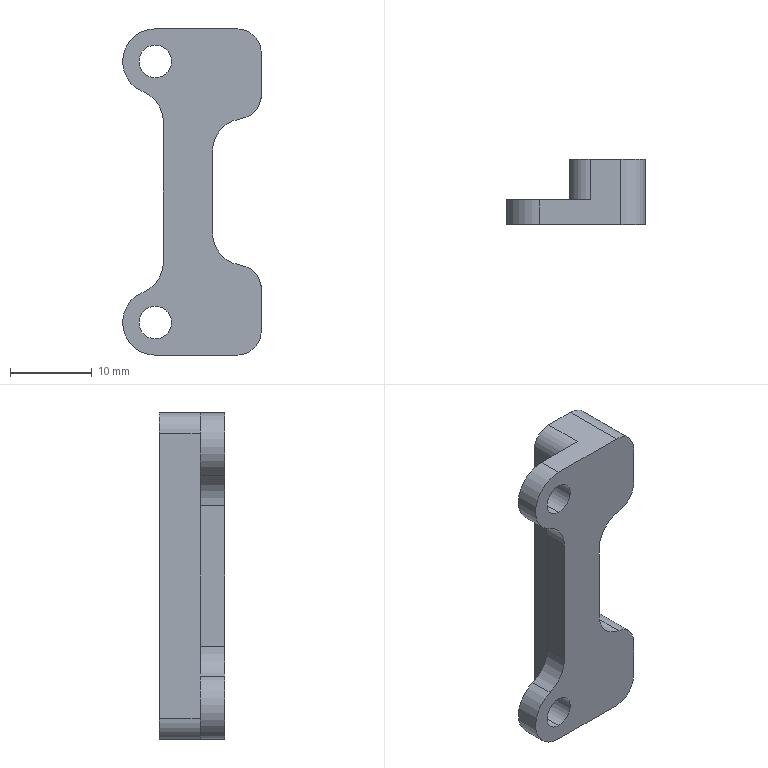NC program | Mastercam | posted with a generic post | part box 17 x 8 x 40 mm
Lines 25 to 1287 of 8055:
(8 FEM |TOOL - 8|DIA. OFF. - 8|LEN. - 8|TOOL DIA. - 8.)
N134 T8 M6
N136 G0 G54 G90 X-27.234 Y-18.253 C0. B0. S7000 M3
N138 G43 H8 Z50.
N140 Z3.
N142 G1 Z-8.25 F600.
N144 X-27.475 Y-17.573 Z-8.368 F3000.
N146 G3 X-27.899 Y-16.899 Z-8.5 I-1.697 J-.599
N148 G1 X-28.108 Y-16.578
N150 X-28.311 Y-16.174
N152 X-28.477 Y-15.79
N154 X-28.607 Y-15.435
N156 X-28.705 Y-15.109
N158 X-28.778 Y-14.809
N160 X-28.832 Y-14.534
N162 X-28.872 Y-14.281
N164 X-28.925 Y-13.837
N166 X-28.957 Y-13.437
N168 X-28.976 Y-13.068
N170 X-28.987 Y-12.722
N172 X-28.993 Y-12.392
N174 X-28.997 Y-12.073
N176 X-28.998 Y-11.761
N178 Y-11.455
N180 X-28.997 Y-11.151
N182 X-28.996 Y-10.85
N184 X-28.995 Y-10.55
N186 X-28.993 Y-10.251
N188 X-28.991 Y-9.952
N190 X-28.989 Y-9.653
N192 X-28.987 Y-9.355
N194 X-28.985 Y-9.056
N196 X-28.983 Y-8.757
N198 X-28.981 Y-8.459
N200 X-28.979 Y-8.16
N202 X-28.977 Y-7.862
N204 X-28.975 Y-7.563
N206 X-28.973 Y-7.264
N208 X-28.971 Y-6.965
N210 X-28.969 Y-6.666
N212 X-28.967 Y-6.367
N214 X-28.965 Y-6.068
N216 X-28.963 Y-5.769
N218 X-28.961 Y-5.47
N220 X-28.958 Y-5.171
N222 X-28.956 Y-4.872
N224 X-28.954 Y-4.573
N226 X-28.952 Y-4.273
N228 X-28.95 Y-3.974
N230 X-28.948 Y-3.674
N232 X-28.946 Y-3.375
N234 X-28.944 Y-3.075
N236 X-28.942 Y-2.776
N238 X-28.94 Y-2.476
N240 X-28.938 Y-2.176
N242 X-28.936 Y-1.877
N244 X-28.934 Y-1.577
N246 X-28.932 Y-1.277
N248 X-28.93 Y-.977
N250 X-28.928 Y-.677
N252 X-28.926 Y-.377
N254 X-28.924 Y-.077
N256 X-28.921 Y.223
N258 X-28.919 Y.523
N260 X-28.917 Y.823
N262 X-28.915 Y1.123
N264 X-28.913 Y1.423
N266 X-28.911 Y1.724
N268 X-28.909 Y2.024
N270 X-28.907 Y2.324
N272 X-28.905 Y2.625
N274 X-28.903 Y2.925
N276 X-28.901 Y3.225
N278 X-28.899 Y3.526
N280 X-28.897 Y3.826
N282 X-28.895 Y4.127
N284 X-28.893 Y4.428
N286 X-28.891 Y4.728
N288 X-28.888 Y5.029
N290 X-28.886 Y5.329
N292 X-28.884 Y5.63
N294 X-28.882 Y5.931
N296 X-28.88 Y6.232
N298 X-28.878 Y6.532
N300 X-28.876 Y6.833
N302 X-28.874 Y7.134
N304 X-28.872 Y7.435
N306 X-28.87 Y7.736
N308 X-28.868 Y8.037
N310 X-28.866 Y8.338
N312 X-28.864 Y8.639
N314 X-28.862 Y8.94
N316 X-28.86 Y9.241
N318 X-28.858 Y9.542
N320 X-28.855 Y9.843
N322 X-28.853 Y10.144
N324 X-28.851 Y10.445
N326 X-28.849 Y10.746
N328 X-28.847 Y11.047
N330 X-28.845 Y11.348
N332 X-28.843 Y11.65
N334 X-28.841 Y11.951
N336 X-28.839 Y12.252
N338 X-28.837 Y12.554
N340 X-28.829 Y12.843
N342 X-28.792 Y13.204
N344 X-28.72 Y13.565
N346 X-28.614 Y13.921
N348 X-28.475 Y14.267
N350 X-28.308 Y14.598
N352 X-28.116 Y14.911
N354 X-27.903 Y15.204
N356 X-27.674 Y15.473
N358 X-27.432 Y15.72
N360 X-27.181 Y15.944
N362 X-26.925 Y16.145
N364 X-26.666 Y16.326
N366 X-26.408 Y16.487
N368 X-26.15 Y16.629
N370 X-25.896 Y16.756
N372 X-25.646 Y16.867
N374 X-25.401 Y16.966
N376 X-25.161 Y17.052
N378 X-24.926 Y17.128
N380 X-24.697 Y17.195
N382 X-24.263 Y17.305
N384 X-23.847 Y17.392
N386 X-23.447 Y17.46
N388 X-23.062 Y17.514
N390 X-22.69 Y17.556
N392 X-22.329 Y17.59
N394 X-21.978 Y17.617
N396 X-21.635 Y17.638
N398 X-21.299 Y17.654
N400 X-20.968 Y17.667
N402 X-20.643 Y17.678
N404 X-20.322 Y17.685
N406 X-20.004 Y17.691
N408 X-19.689 Y17.696
N410 X-19.377 Y17.699
N412 X-19.066 Y17.701
N414 X-18.757 Y17.702
N416 X-18.449
N418 X-18.143
N420 X-17.837
N422 X-17.533 Y17.701
N424 X-17.228 Y17.7
N426 X-16.924 Y17.698
N428 X-16.621 Y17.697
N430 X-16.317 Y17.695
N432 X-16.014 Y17.693
N434 X-15.711 Y17.692
N436 X-15.408 Y17.69
N438 X-15.105 Y17.688
N440 X-14.803 Y17.686
N442 X-14.5 Y17.684
N444 X-14.197 Y17.682
N446 X-13.895 Y17.68
N448 X-13.592 Y17.678
N450 X-13.289 Y17.676
N452 X-12.987 Y17.674
N454 X-12.684 Y17.672
N456 X-12.381 Y17.67
N458 X-12.079 Y17.668
N460 X-11.776 Y17.665
N462 X-11.473 Y17.663
N464 X-11.171 Y17.661
N466 X-10.868 Y17.659
N468 X-10.565 Y17.657
N470 X-10.263 Y17.655
N472 X-9.96 Y17.653
N474 X-9.657 Y17.651
N476 X-9.354 Y17.649
N478 X-9.052 Y17.647
N480 X-8.749 Y17.645
N482 X-8.446 Y17.643
N484 X-8.143 Y17.641
N486 X-7.841 Y17.638
N488 X-7.538 Y17.636
N490 X-7.235 Y17.634
N492 X-6.932 Y17.632
N494 X-6.629 Y17.63
N496 X-6.327 Y17.628
N498 X-6.024 Y17.626
N500 X-5.721 Y17.624
N502 X-5.418 Y17.622
N504 X-5.115 Y17.62
N506 X-4.812 Y17.618
N508 X-4.509 Y17.616
N510 X-4.206 Y17.614
N512 X-3.903 Y17.612
N514 X-3.599 Y17.61
N516 X-3.295 Y17.608
N518 X-2.99 Y17.607
N520 X-2.685 Y17.606
N522 X-2.38 Y17.605
N524 X-2.075 Y17.604
N526 X-1.769
N528 X-1.463 Y17.603
N530 X-1.157
N532 X-.851 Y17.602
N534 X-.545
N536 X-.239
N538 X.067 Y17.601
N540 X.374
N542 X.68
N544 X.986
N546 X1.293
N548 X1.6
N550 X1.906
N552 X2.213 Y17.6
N554 X2.519
N556 X2.826
N558 X3.133
N560 X3.439
N562 X3.746
N564 X4.053
N566 X4.359
N568 X4.666
N570 X4.973
N572 X5.279
N574 X5.586
N576 X5.893
N578 X6.199
N580 X6.506
N582 X6.813
N584 X7.12
N586 X7.426
N588 X7.733
N590 X8.04
N592 X8.346
N594 X8.653
N596 X8.96
N598 X9.267
N600 X9.573
N602 X9.88
N604 X10.187
N606 X10.493
N608 X10.8
N610 X11.107
N612 X11.414
N614 X11.72
N616 X12.027
N618 X12.334
N620 X12.641
N622 X12.947
N624 X13.254
N626 X13.561
N628 X13.867
N630 X14.174
N632 X14.481
N634 X14.788
N636 X15.094
N638 X15.401
N640 X15.708
N642 X16.015
N644 X16.321
N646 X16.628
N648 X16.935
N650 X17.241
N652 X17.548
N654 X17.855
N656 X18.162
N658 X18.468
N660 X18.775
N662 X19.082
N664 X19.389
N666 X19.695
N668 X20.002
N670 X20.309
N672 X20.616
N674 X20.922
N676 X21.229
N678 X21.536
N680 X21.842
N682 X22.149
N684 X22.456
N686 X22.763
N688 X23.07
N690 X23.335 Y17.595
N692 X23.605 Y17.572
N694 X23.881 Y17.527
N696 X24.16 Y17.461
N698 X24.439 Y17.374
N700 X24.714 Y17.266
N702 X24.984 Y17.138
N704 X25.246 Y16.992
N706 X25.497 Y16.83
N708 X25.737 Y16.653
N710 X25.965 Y16.463
N712 X26.179 Y16.263
N714 X26.38 Y16.054
N716 X26.567 Y15.839
N718 X26.74 Y15.619
N720 X26.901 Y15.395
N722 X27.048 Y15.168
N724 X27.183 Y14.941
N726 X27.308 Y14.713
N728 X27.421 Y14.487
N730 X27.525 Y14.261
N732 X27.619 Y14.037
N734 X27.705 Y13.816
N736 X27.852 Y13.388
N738 X27.975 Y12.971
N740 X28.076 Y12.564
N742 X28.161 Y12.168
N744 X28.231 Y11.782
N746 X28.29 Y11.405
N748 X28.339 Y11.037
N750 X28.38 Y10.677
N752 X28.414 Y10.324
N754 X28.443 Y9.978
N756 X28.467 Y9.637
N758 X28.487 Y9.3
N760 X28.504 Y8.968
N762 X28.519 Y8.639
N764 X28.531 Y8.314
N766 X28.541 Y7.991
N768 X28.55 Y7.67
N770 X28.557 Y7.351
N772 X28.564 Y7.035
N774 X28.569 Y6.719
N776 X28.574 Y6.405
N778 X28.578 Y6.092
N780 X28.581 Y5.78
N782 X28.584 Y5.468
N784 X28.586 Y5.158
N786 X28.588 Y4.848
N788 X28.59 Y4.538
N790 X28.591 Y4.229
N792 X28.593 Y3.92
N794 X28.594 Y3.611
N796 X28.595 Y3.303
N798 Y2.995
N800 X28.596 Y2.687
N802 X28.597 Y2.38
N804 Y2.072
N806 X28.598 Y1.765
N808 Y1.457
N810 Y1.15
N812 X28.599 Y.843
N814 Y.536
N816 Y.229
N818 Y-.078
N820 Y-.385
N822 Y-.692
N824 Y-.999
N826 X28.6 Y-1.306
N828 Y-1.613
N830 Y-1.92
N832 Y-2.226
N834 Y-2.533
N836 Y-2.84
N838 Y-3.147
N840 Y-3.454
N842 Y-3.76
N844 Y-4.067
N846 Y-4.374
N848 Y-4.681
N850 Y-4.987
N852 Y-5.294
N854 Y-5.601
N856 Y-5.908
N858 Y-6.214
N860 Y-6.521
N862 Y-6.828
N864 Y-7.135
N866 Y-7.441
N868 Y-7.748
N870 Y-8.055
N872 Y-8.361
N874 Y-8.668
N876 Y-8.975
N878 Y-9.282
N880 Y-9.588
N882 Y-9.895
N884 Y-10.202
N886 Y-10.509
N888 Y-10.815
N890 Y-11.122
N892 Y-11.429
N894 Y-11.736
N896 Y-12.042
N898 X28.597 Y-12.286
N900 X28.577 Y-12.558
N902 X28.536 Y-12.834
N904 X28.474 Y-13.112
N906 X28.391 Y-13.391
N908 X28.286 Y-13.667
N910 X28.161 Y-13.938
N912 X28.018 Y-14.201
N914 X27.859 Y-14.455
N916 X27.684 Y-14.697
N918 X27.497 Y-14.927
N920 X27.298 Y-15.143
N922 X27.091 Y-15.346
N924 X26.877 Y-15.536
N926 X26.657 Y-15.711
N928 X26.433 Y-15.874
N930 X26.207 Y-16.024
N932 X25.98 Y-16.161
N934 X25.753 Y-16.287
N936 X25.526 Y-16.402
N938 X25.3 Y-16.507
N940 X25.076 Y-16.603
N942 X24.854 Y-16.691
N944 X24.425 Y-16.84
N946 X24.007 Y-16.965
N948 X23.599 Y-17.068
N950 X23.202 Y-17.154
N952 X22.815 Y-17.226
N954 X22.438 Y-17.285
N956 X22.069 Y-17.335
N958 X21.709 Y-17.376
N960 X21.355 Y-17.411
N962 X21.008 Y-17.44
N964 X20.666 Y-17.465
N966 X20.329 Y-17.485
N968 X19.997 Y-17.503
N970 X19.668 Y-17.517
N972 X19.342 Y-17.53
N974 X19.019 Y-17.54
N976 X18.698 Y-17.549
N978 X18.379 Y-17.557
N980 X18.062 Y-17.563
N982 X17.747 Y-17.569
N984 X17.433 Y-17.573
N986 X17.119 Y-17.577
N988 X16.807 Y-17.581
N990 X16.496 Y-17.584
N992 X16.185 Y-17.586
N994 X15.875 Y-17.588
N996 X15.565 Y-17.59
N998 X15.256 Y-17.591
N1000 X14.947 Y-17.593
N1002 X14.638 Y-17.594
N1004 X14.33 Y-17.595
N1006 X14.022
N1008 X13.714 Y-17.596
N1010 X13.407 Y-17.597
N1012 X13.099
N1014 X12.792 Y-17.598
N1016 X12.484
N1018 X12.177
N1020 X11.87
N1022 X11.563 Y-17.599
N1024 X11.256
N1026 X10.949
N1028 X10.642
N1030 X10.335
N1032 X10.028
N1034 X9.721 Y-17.6
N1036 X9.414
N1038 X9.107
N1040 X8.801
N1042 X8.494
N1044 X8.187
N1046 X7.88
N1048 X7.573
N1050 X7.267
N1052 X6.96
N1054 X6.653
N1056 X6.346
N1058 X6.04
N1060 X5.733
N1062 X5.426
N1064 X5.119
N1066 X4.813
N1068 X4.506
N1070 X4.199
N1072 X3.892
N1074 X3.586
N1076 X3.279
N1078 X2.972
N1080 X2.665
N1082 X2.359
N1084 X2.052
N1086 X1.745
N1088 X1.439
N1090 X1.132
N1092 X.825
N1094 X.518
N1096 X.212
N1098 X-.095
N1100 X-.402
N1102 X-.709
N1104 X-1.015
N1106 X-1.322
N1108 X-1.629
N1110 X-1.936
N1112 X-2.242
N1114 X-2.549
N1116 X-2.856
N1118 X-3.162
N1120 X-3.469
N1122 X-3.776
N1124 X-4.083
N1126 X-4.389
N1128 X-4.696
N1130 X-5.003
N1132 X-5.31
N1134 X-5.616
N1136 X-5.923
N1138 X-6.23
N1140 X-6.536
N1142 X-6.843
N1144 X-7.15
N1146 X-7.457
N1148 X-7.763
N1150 X-8.07
N1152 X-8.377
N1154 X-8.684
N1156 X-8.99
N1158 X-9.297
N1160 X-9.604
N1162 X-9.91
N1164 X-10.217
N1166 X-10.524
N1168 X-10.831
N1170 X-11.137
N1172 X-11.444
N1174 X-11.751
N1176 X-12.058
N1178 X-12.364
N1180 X-12.671
N1182 X-12.978
N1184 X-13.284
N1186 X-13.591
N1188 X-13.898
N1190 X-14.205
N1192 X-14.511
N1194 X-14.818
N1196 X-15.125
N1198 X-15.432
N1200 X-15.738
N1202 X-16.045
N1204 X-16.352
N1206 X-16.658
N1208 X-16.965
N1210 X-17.272
N1212 X-17.579
N1214 X-17.885
N1216 X-18.192
N1218 X-18.499
N1220 X-18.806
N1222 X-19.112
N1224 X-19.419
N1226 X-19.726
N1228 X-20.033
N1230 X-20.339
N1232 X-20.646
N1234 X-20.953
N1236 X-21.259
N1238 X-21.566
N1240 X-21.873
N1242 X-22.18
N1244 X-22.486
N1246 X-22.793
N1248 X-22.993 Y-17.599
N1250 X-23.283 Y-17.582
N1252 X-23.573 Y-17.543
N1254 X-23.86 Y-17.485
N1256 X-24.146 Y-17.405
N1258 X-24.427 Y-17.306
N1260 X-24.702 Y-17.187
N1262 X-24.969 Y-17.051
N1264 X-25.226 Y-16.898
N1266 X-25.473 Y-16.73
N1268 X-25.708 Y-16.549
N1270 X-25.93 Y-16.357
N1272 X-26.139 Y-16.154
N1274 X-26.335 Y-15.944
N1276 X-26.517 Y-15.728
N1278 X-26.686 Y-15.507
N1280 X-26.842 Y-15.282
N1282 X-26.986 Y-15.055
N1284 X-27.118 Y-14.828
N1286 X-27.24 Y-14.6
N1288 X-27.35 Y-14.373
N1290 X-27.451 Y-14.147
N1292 X-27.543 Y-13.924
N1294 X-27.627 Y-13.702
N1296 X-27.77 Y-13.274
N1298 X-27.889 Y-12.856
N1300 X-27.987 Y-12.449
N1302 X-28.069 Y-12.053
N1304 X-28.136 Y-11.667
N1306 X-28.192 Y-11.29
N1308 X-28.238 Y-10.922
N1310 X-28.276 Y-10.562
N1312 X-28.308 Y-10.21
N1314 X-28.334 Y-9.863
N1316 X-28.356 Y-9.522
N1318 X-28.374 Y-9.185
N1320 X-28.388 Y-8.853
N1322 X-28.4 Y-8.524
N1324 X-28.41 Y-8.198
N1326 X-28.419 Y-7.876
N1328 X-28.425 Y-7.555
N1330 X-28.43 Y-7.236
N1332 X-28.434 Y-6.919
N1334 X-28.438 Y-6.604
N1336 X-28.44 Y-6.29
N1338 X-28.442 Y-5.977
N1340 X-28.443 Y-5.665
N1342 X-28.444 Y-5.353
N1344 Y-5.043
N1346 Y-4.733
N1348 X-28.443 Y-4.423
N1350 Y-4.114
N1352 X-28.442 Y-3.805
N1354 X-28.441 Y-3.496
N1356 X-28.44 Y-3.188
N1358 X-28.438 Y-2.88
N1360 X-28.437 Y-2.572
N1362 X-28.435 Y-2.265
N1364 X-28.434 Y-1.957
N1366 X-28.432 Y-1.65
N1368 X-28.43 Y-1.342
N1370 X-28.428 Y-1.035
N1372 X-28.426 Y-.728
N1374 X-28.425 Y-.421
N1376 X-28.423 Y-.114
N1378 X-28.421 Y.193
N1380 X-28.419 Y.5
N1382 X-28.417 Y.807
N1384 X-28.415 Y1.114
N1386 X-28.413 Y1.421
N1388 X-28.411 Y1.728
N1390 X-28.409 Y2.034
N1392 X-28.407 Y2.341
N1394 X-28.405 Y2.648
N1396 X-28.402 Y2.955
N1398 X-28.4 Y3.262
N1400 X-28.398 Y3.568
N1402 X-28.396 Y3.875
N1404 X-28.394 Y4.182
N1406 X-28.392 Y4.489
N1408 X-28.39 Y4.795
N1410 X-28.388 Y5.102
N1412 X-28.386 Y5.409
N1414 X-28.384 Y5.716
N1416 X-28.382 Y6.022
N1418 X-28.379 Y6.329
N1420 X-28.377 Y6.636
N1422 X-28.375 Y6.943
N1424 X-28.373 Y7.249
N1426 X-28.371 Y7.556
N1428 X-28.369 Y7.863
N1430 X-28.367 Y8.169
N1432 X-28.365 Y8.476
N1434 X-28.363 Y8.783
N1436 X-28.361 Y9.09
N1438 X-28.358 Y9.396
N1440 X-28.356 Y9.703
N1442 X-28.354 Y10.01
N1444 X-28.352 Y10.317
N1446 X-28.35 Y10.625
N1448 X-28.347 Y10.838
N1450 X-28.333 Y11.114
N1452 X-28.305 Y11.399
N1454 X-28.262 Y11.687
N1456 X-28.203 Y11.974
N1458 X-28.127 Y12.258
N1460 X-28.036 Y12.537
N1462 X-27.93 Y12.81
N1464 X-27.809 Y13.077
N1466 X-27.674 Y13.335
N1468 X-27.526 Y13.585
N1470 X-27.368 Y13.824
N1472 X-27.198 Y14.054
N1474 X-27.019 Y14.273
N1476 X-26.831 Y14.481
N1478 X-26.637 Y14.678
N1480 X-26.436 Y14.864
N1482 X-26.231 Y15.039
N1484 X-26.021 Y15.203
N1486 X-25.809 Y15.356
N1488 X-25.594 Y15.5
N1490 X-25.377 Y15.633
N1492 X-25.16 Y15.757
N1494 X-24.942 Y15.872
N1496 X-24.725 Y15.978
N1498 X-24.509 Y16.077
N1500 X-24.087 Y16.249
N1502 X-23.67 Y16.396
N1504 X-23.261 Y16.521
N1506 X-22.859 Y16.628
N1508 X-22.465 Y16.717
N1510 X-22.08 Y16.793
N1512 X-21.702 Y16.857
N1514 X-21.331 Y16.911
N1516 X-20.968 Y16.957
N1518 X-20.611 Y16.995
N1520 X-20.26 Y17.027
N1522 X-19.915 Y17.054
N1524 X-19.574 Y17.077
N1526 X-19.238 Y17.096
N1528 X-18.905 Y17.111
N1530 X-18.576 Y17.124
N1532 X-18.25 Y17.135
N1534 X-17.926 Y17.144
N1536 X-17.605 Y17.151
N1538 X-17.286 Y17.157
N1540 X-16.969 Y17.161
N1542 X-16.653 Y17.165
N1544 X-16.338 Y17.168
N1546 X-16.024 Y17.17
N1548 X-15.712 Y17.171
N1550 X-15.4 Y17.172
N1552 X-15.089 Y17.173
N1554 X-14.779
N1556 X-14.469
N1558 X-14.159 Y17.172
N1560 X-13.85
N1562 X-13.542 Y17.171
N1564 X-13.233 Y17.17
N1566 X-12.925 Y17.168
N1568 X-12.617 Y17.167
N1570 X-12.309 Y17.165
N1572 X-12.002 Y17.164
N1574 X-11.694 Y17.162
N1576 X-11.387 Y17.161
N1578 X-11.08 Y17.159
N1580 X-10.772 Y17.157
N1582 X-10.465 Y17.155
N1584 X-10.158 Y17.153
N1586 X-9.851 Y17.151
N1588 X-9.544 Y17.149
N1590 X-9.237 Y17.147
N1592 X-8.93 Y17.145
N1594 X-8.623 Y17.143
N1596 X-8.317 Y17.141
N1598 X-8.01 Y17.139
N1600 X-7.703 Y17.137
N1602 X-7.396 Y17.135
N1604 X-7.089 Y17.133
N1606 X-6.782 Y17.131
N1608 X-6.476 Y17.129
N1610 X-6.169 Y17.127
N1612 X-5.862 Y17.125
N1614 X-5.556 Y17.123
N1616 X-5.25 Y17.121
N1618 X-4.945 Y17.119
N1620 X-4.639 Y17.117
N1622 X-4.334 Y17.115
N1624 X-4.028 Y17.114
N1626 X-3.723 Y17.112
N1628 X-3.417 Y17.111
N1630 X-3.112 Y17.11
N1632 X-2.806 Y17.109
N1634 X-2.5 Y17.108
N1636 X-2.195 Y17.107
N1638 X-1.889 Y17.106
N1640 X-1.583
N1642 X-1.277 Y17.105
N1644 X-.971 Y17.104
N1646 X-.665
N1648 X-.359 Y17.103
N1650 X-.052
N1652 X.254
N1654 X.56 Y17.102
N1656 X.866
N1658 X1.173
N1660 X1.479
N1662 X1.786 Y17.101
N1664 X2.092
N1666 X2.399
N1668 X2.705
N1670 X3.012
N1672 X3.318
N1674 X3.625
N1676 X3.932
N1678 X4.238 Y17.1
N1680 X4.545
N1682 X4.852
N1684 X5.158
N1686 X5.465
N1688 X5.772
N1690 X6.078
N1692 X6.385
N1694 X6.692
N1696 X6.998
N1698 X7.305
N1700 X7.612
N1702 X7.919
N1704 X8.225
N1706 X8.532
N1708 X8.839
N1710 X9.145
N1712 X9.452
N1714 X9.759
N1716 X10.066
N1718 X10.372
N1720 X10.679
N1722 X10.986
N1724 X11.292
N1726 X11.599
N1728 X11.906
N1730 X12.213
N1732 X12.519
N1734 X12.826
N1736 X13.133
N1738 X13.439
N1740 X13.746
N1742 X14.053
N1744 X14.36
N1746 X14.666
N1748 X14.973
N1750 X15.28
N1752 X15.587
N1754 X15.893
N1756 X16.2
N1758 X16.507
N1760 X16.813
N1762 X17.12
N1764 X17.427
N1766 X17.734
N1768 X18.04
N1770 X18.347
N1772 X18.654
N1774 X18.961
N1776 X19.267
N1778 X19.574
N1780 X19.881
N1782 X20.187
N1784 X20.494
N1786 X20.801
N1788 X21.108
N1790 X21.319 Y17.099
N1792 X21.591 Y17.088
N1794 X21.872 Y17.063
N1796 X22.155 Y17.025
N1798 X22.438 Y16.971
N1800 X22.72 Y16.903
N1802 X22.997 Y16.82
N1804 X23.269 Y16.723
N1806 X23.535 Y16.612
N1808 X23.794 Y16.489
N1810 X24.045 Y16.352
N1812 X24.287 Y16.205
N1814 X24.521 Y16.047
N1816 X24.744 Y15.881
N1818 X24.958 Y15.705
N1820 X25.161 Y15.523
N1822 X25.355 Y15.334
N1824 X25.538 Y15.139
N1826 X25.712 Y14.94
N1828 X25.875 Y14.737
N1830 X26.029 Y14.531
N1832 X26.174 Y14.323
N1834 X26.309 Y14.113
N1836 X26.436 Y13.902
N1838 X26.554 Y13.69
N1840 X26.665 Y13.478
N1842 X26.86 Y13.064
N1844 X27.03 Y12.652
N1846 X27.177 Y12.245
N1848 X27.305 Y11.844
N1850 X27.414 Y11.449
N1852 X27.509 Y11.061
N1854 X27.59 Y10.68
N1856 X27.66 Y10.306
N1858 X27.72 Y9.938
N1860 X27.772 Y9.576
N1862 X27.817 Y9.22
N1864 X27.855 Y8.869
N1866 X27.888 Y8.524
N1868 X27.917 Y8.182
N1870 X27.942 Y7.845
N1872 X27.963 Y7.511
N1874 X27.982 Y7.18
N1876 X27.998 Y6.853
N1878 X28.011 Y6.527
N1880 X28.023 Y6.205
N1882 X28.034 Y5.884
N1884 X28.042 Y5.564
N1886 X28.05 Y5.247
N1888 X28.057 Y4.931
N1890 X28.063 Y4.616
N1892 X28.068 Y4.302
N1894 X28.072 Y3.989
N1896 X28.076 Y3.676
N1898 X28.079 Y3.365
N1900 X28.082 Y3.054
N1902 X28.084 Y2.744
N1904 X28.086 Y2.434
N1906 X28.088 Y2.124
N1908 X28.09 Y1.815
N1910 X28.091 Y1.506
N1912 X28.092 Y1.198
N1914 X28.093 Y.89
N1916 X28.094 Y.581
N1918 X28.095 Y.274
N1920 X28.096 Y-.034
N1922 Y-.342
N1924 X28.097 Y-.649
N1926 Y-.957
N1928 X28.098 Y-1.264
N1930 Y-1.571
N1932 Y-1.878
N1934 Y-2.185
N1936 X28.099 Y-2.492
N1938 Y-2.799
N1940 Y-3.106
N1942 Y-3.413
N1944 Y-3.72
N1946 Y-4.027
N1948 Y-4.334
N1950 X28.1 Y-4.641
N1952 Y-4.948
N1954 Y-5.255
N1956 Y-5.561
N1958 Y-5.868
N1960 Y-6.175
N1962 Y-6.482
N1964 Y-6.788
N1966 Y-7.095
N1968 Y-7.402
N1970 Y-7.709
N1972 Y-8.016
N1974 Y-8.322
N1976 Y-8.629
N1978 Y-8.936
N1980 Y-9.243
N1982 Y-9.549
N1984 Y-9.856
N1986 Y-10.164
N1988 X28.096 Y-10.416
N1990 X28.08 Y-10.692
N1992 X28.051 Y-10.974
N1994 X28.007 Y-11.257
N1996 X27.949 Y-11.54
N1998 X27.875 Y-11.82
N2000 X27.787 Y-12.095
N2002 X27.685 Y-12.365
N2004 X27.569 Y-12.629
N2006 X27.441 Y-12.885
N2008 X27.3 Y-13.134
N2010 X27.15 Y-13.372
N2012 X26.988 Y-13.602
N2014 X26.818 Y-13.822
N2016 X26.641 Y-14.032
N2018 X26.455 Y-14.232
N2020 X26.265 Y-14.422
N2022 X26.068 Y-14.602
N2024 X25.868 Y-14.772
N2026 X25.663 Y-14.932
N2028 X25.457 Y-15.082
N2030 X25.247 Y-15.224
N2032 X25.037 Y-15.355
N2034 X24.826 Y-15.479
N2036 X24.614 Y-15.595
N2038 X24.402 Y-15.703
N2040 X23.988 Y-15.893
N2042 X23.577 Y-16.059
N2044 X23.171 Y-16.202
N2046 X22.771 Y-16.326
N2048 X22.378 Y-16.433
N2050 X21.991 Y-16.524
N2052 X21.611 Y-16.604
N2054 X21.238 Y-16.672
N2056 X20.871 Y-16.73
N2058 X20.51 Y-16.781
N2060 X20.156 Y-16.824
N2062 X19.806 Y-16.862
N2064 X19.461 Y-16.894
N2066 X19.12 Y-16.922
N2068 X18.784 Y-16.946
N2070 X18.45 Y-16.967
N2072 X18.12 Y-16.985
N2074 X17.793 Y-17.
N2076 X17.468 Y-17.014
N2078 X17.146 Y-17.025
N2080 X16.825 Y-17.035
N2082 X16.506 Y-17.044
N2084 X16.189 Y-17.051
N2086 X15.873 Y-17.058
N2088 X15.558 Y-17.064
N2090 X15.244 Y-17.068
N2092 X14.932 Y-17.073
N2094 X14.62 Y-17.076
N2096 X14.308 Y-17.08
N2098 X13.997 Y-17.082
N2100 X13.687 Y-17.085
N2102 X13.377 Y-17.087
N2104 X13.068 Y-17.089
N2106 X12.759 Y-17.09
N2108 X12.45 Y-17.091
N2110 X12.142 Y-17.093
N2112 X11.833 Y-17.094
N2114 X11.525
N2116 X11.217 Y-17.095
N2118 X10.91 Y-17.096
N2120 X10.602
N2122 X10.295 Y-17.097
N2124 X9.987
N2126 X9.68 Y-17.098
N2128 X9.373
N2130 X9.066
N2132 X8.759 Y-17.099
N2134 X8.451
N2136 X8.144
N2138 X7.838
N2140 X7.531
N2142 X7.224
N2144 X6.917
N2146 X6.61
N2148 X6.303 Y-17.1
N2150 X5.996
N2152 X5.689
N2154 X5.383
N2156 X5.076
N2158 X4.769
N2160 X4.462
N2162 X4.156
N2164 X3.849
N2166 X3.542
N2168 X3.235
N2170 X2.928
N2172 X2.622
N2174 X2.315
N2176 X2.008
N2178 X1.701
N2180 X1.395
N2182 X1.088
N2184 X.781
N2186 X.475
N2188 X.168
N2190 X-.139
N2192 X-.446
N2194 X-.752
N2196 X-1.059
N2198 X-1.366
N2200 X-1.673
N2202 X-1.979
N2204 X-2.286
N2206 X-2.593
N2208 X-2.9
N2210 X-3.206
N2212 X-3.513
N2214 X-3.82
N2216 X-4.126
N2218 X-4.433
N2220 X-4.74
N2222 X-5.047
N2224 X-5.353
N2226 X-5.66
N2228 X-5.967
N2230 X-6.274
N2232 X-6.58
N2234 X-6.887
N2236 X-7.194
N2238 X-7.5
N2240 X-7.807
N2242 X-8.114
N2244 X-8.421
N2246 X-8.727
N2248 X-9.034
N2250 X-9.341
N2252 X-9.648
N2254 X-9.954
N2256 X-10.261
N2258 X-10.568
N2260 X-10.874
N2262 X-11.181
N2264 X-11.488
N2266 X-11.795
N2268 X-12.101
N2270 X-12.408
N2272 X-12.715
N2274 X-13.022
N2276 X-13.328
N2278 X-13.635
N2280 X-13.942
N2282 X-14.248
N2284 X-14.555
N2286 X-14.862
N2288 X-15.169
N2290 X-15.475
N2292 X-15.782
N2294 X-16.089
N2296 X-16.396
N2298 X-16.702
N2300 X-17.009
N2302 X-17.316
N2304 X-17.622
N2306 X-17.929
N2308 X-18.236
N2310 X-18.543
N2312 X-18.849
N2314 X-19.156
N2316 X-19.463
N2318 X-19.77
N2320 X-20.076
N2322 X-20.383
N2324 X-20.69
N2326 X-21.01
N2328 X-21.255 Y-17.095
N2330 X-21.524 Y-17.08
N2332 X-21.802 Y-17.053
N2334 X-22.082 Y-17.011
N2336 X-22.363 Y-16.955
N2338 X-22.642 Y-16.884
N2340 X-22.917 Y-16.799
N2342 X-23.187 Y-16.7
N2344 X-23.452 Y-16.588
N2346 X-23.709 Y-16.463
N2348 X-23.958 Y-16.326
N2350 X-24.2 Y-16.177
N2352 X-24.431 Y-16.019
N2354 X-24.653 Y-15.851
N2356 X-24.866 Y-15.675
N2358 X-25.068 Y-15.493
N2360 X-25.261 Y-15.303
N2362 X-25.443 Y-15.108
N2364 X-25.616 Y-14.908
N2366 X-25.778 Y-14.705
N2368 X-25.932 Y-14.498
N2370 X-26.075 Y-14.29
N2372 X-26.21 Y-14.079
N2374 X-26.336 Y-13.868
N2376 X-26.454 Y-13.656
N2378 X-26.563 Y-13.444
N2380 X-26.757 Y-13.029
N2382 X-26.926 Y-12.616
N2384 X-27.072 Y-12.208
N2386 X-27.198 Y-11.805
N2388 X-27.306 Y-11.409
N2390 X-27.399 Y-11.02
N2392 X-27.478 Y-10.638
N2394 X-27.547 Y-10.263
N2396 X-27.605 Y-9.894
N2398 X-27.655 Y-9.532
N2400 X-27.698 Y-9.175
N2402 X-27.735 Y-8.824
N2404 X-27.766 Y-8.477
N2406 X-27.793 Y-8.135
N2408 X-27.816 Y-7.797
N2410 X-27.835 Y-7.463
N2412 X-27.852 Y-7.132
N2414 X-27.865 Y-6.804
N2416 X-27.877 Y-6.478
N2418 X-27.887 Y-6.155
N2420 X-27.895 Y-5.834
N2422 X-27.902 Y-5.515
N2424 X-27.908 Y-5.197
N2426 X-27.913 Y-4.88
N2428 X-27.916 Y-4.565
N2430 X-27.919 Y-4.251
N2432 X-27.921 Y-3.938
N2434 X-27.923 Y-3.626
N2436 X-27.924 Y-3.314
N2438 X-27.925 Y-3.003
N2440 Y-2.693
N2442 Y-2.383
N2444 Y-2.073
N2446 Y-1.764
N2448 X-27.924 Y-1.455
N2450 X-27.923 Y-1.147
N2452 X-27.922 Y-.838
N2454 X-27.921 Y-.53
N2456 X-27.919 Y-.222
N2458 X-27.918 Y.085
N2460 X-27.917 Y.393
N2462 X-27.915 Y.701
N2464 X-27.913 Y1.008
N2466 X-27.912 Y1.315
N2468 X-27.91 Y1.623
N2470 X-27.908 Y1.93
N2472 X-27.906 Y2.237
N2474 X-27.904 Y2.544
N2476 X-27.902 Y2.851
N2478 X-27.9 Y3.158
N2480 X-27.898 Y3.465
N2482 X-27.896 Y3.772
N2484 X-27.894 Y4.079
N2486 X-27.892 Y4.385
N2488 X-27.89 Y4.692
N2490 X-27.888 Y4.999
N2492 X-27.886 Y5.306
N2494 X-27.884 Y5.613
N2496 X-27.882 Y5.919
N2498 X-27.88 Y6.226
N2500 X-27.878 Y6.533
N2502 X-27.876 Y6.84
N2504 X-27.874 Y7.147
N2506 X-27.872 Y7.453
N2508 X-27.87 Y7.76
N2510 X-27.867 Y8.067
N2512 X-27.865 Y8.374
N2514 X-27.863 Y8.68
N2516 X-27.86 Y9.007
N2518 X-27.85 Y9.407
N2520 X-27.837 Y9.639
N2522 X-27.816 Y9.884
N2524 X-27.785 Y10.14
N2526 X-27.744 Y10.401
N2528 X-27.692 Y10.664
N2530 X-27.628 Y10.929
N2532 X-27.551 Y11.192
N2534 X-27.463 Y11.453
N2536 X-27.364 Y11.71
N2538 X-27.252 Y11.963
N2540 X-27.131 Y12.209
N2542 X-26.998 Y12.45
N2544 X-26.855 Y12.684
N2546 X-26.704 Y12.91
N2548 X-26.544 Y13.128
N2550 X-26.377 Y13.337
N2552 X-26.203 Y13.538
N2554 X-26.023 Y13.73
N2556 X-25.836 Y13.914
N2558 X-25.646 Y14.089
N2560 X-25.451 Y14.255
N2562 X-25.253 Y14.412
N2564 X-25.052 Y14.561
N2566 X-24.849 Y14.702
N2568 X-24.644 Y14.834
N2570 X-24.438 Y14.959
N2572 X-24.231 Y15.077
N2574 X-23.824 Y15.287
N2576 X-23.418 Y15.471
N2578 X-23.013 Y15.633
N2580 X-22.612 Y15.775
N2582 X-22.216 Y15.899
N2584 X-21.825 Y16.006
N2586 X-21.44 Y16.099
N2588 X-21.061 Y16.18
N2590 X-20.688 Y16.249
N2592 X-20.321 Y16.31
N2594 X-19.959 Y16.362
N2596 X-19.603 Y16.407
N2598 X-19.252 Y16.445
N2600 X-18.905 Y16.479
N2602 X-18.563 Y16.507
N2604 X-18.224 Y16.532
N2606 X-17.889 Y16.553
N2608 X-17.557 Y16.571
N2610 X-17.228 Y16.586
N2612 X-16.901 Y16.599
N2614 X-16.577 Y16.61
N2616 X-16.255 Y16.62
N2618 X-15.935 Y16.628
N2620 X-15.616 Y16.634
N2622 X-15.299 Y16.639
N2624 X-14.983 Y16.644
N2626 X-14.668 Y16.647
N2628 X-14.354 Y16.65
N2630 X-14.042 Y16.653
N2632 X-13.729 Y16.654
N2634 X-13.418 Y16.655
N2636 X-13.107 Y16.656
N2638 X-12.797
N2640 X-12.487
N2642 X-12.177
N2644 X-11.868
N2646 X-11.56 Y16.655
N2648 X-11.251 Y16.654
N2650 X-10.943 Y16.653
N2652 X-10.635 Y16.652
N2654 X-10.327 Y16.65
N2656 X-10.019 Y16.649